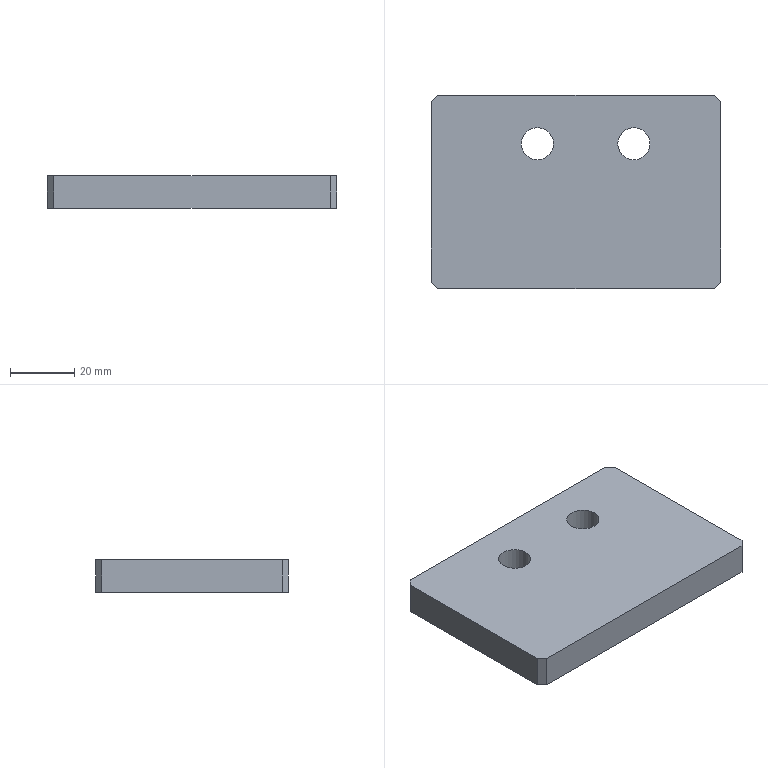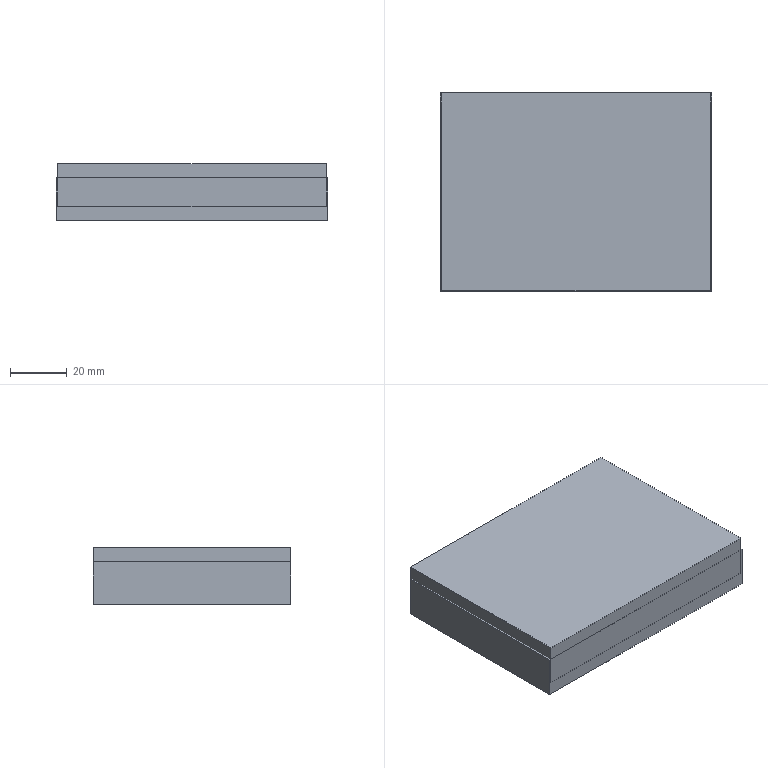CAM job | NX | 3-axis milling, drilling | part box 90 x 60 x 10 mm | stock box 96 x 70 x 20 mm
Tools:
number,name,description,diameter,corner_radius,flute_length,length,flutes
1,D80面刀,,80.0,0.0,50.0,75.0,2
2,D12开粗,,12.0,0.0,50.0,75.0,2
3,D10精光,,10.0,0.0,50.0,75.0,2
5,D6倒角刀,,6.0,0.0,50.0,75.0,2
6,D8.6钻头,,8.6,0.0,50.0,75.0,2
7,M10丝攻,,8.6,0.0,50.0,75.0,2
Operations:
program,operation,operation_type,tool,method,geometry_group,spindle_rpm,surface_speed,feed_per_tooth,feed_cut,feed_plunge,cut_length_mm,path_length_mm,cut_time_min,machine_time_min
G54,PLANAR_MILL,PlanarMilling,D80面刀,METHOD,G54,2000.0,502.0,0.2,800.0,100.0,180.0,215.9,0.225,0.2286
G54,ADAPTIVE_MILLING,CavityMilling,D12开粗,METHOD,WORKPIECE,3000.0,113.0,0.25,1500.0,100.0,3610.156,3666.156,1.991,1.996
G54,PLANAR_MILL_1,PlanarMilling,D10精光,METHOD,WORKPIECE,3000.0,94.0,0.1333,800.0,100.0,694.172,819.237,0.8677,0.8802
G54,SPOT_DRILLING,HoleDrilling,D6倒角刀,METHOD,WORKPIECE,2000.0,37.0,0.0375,150.0,100.0,16.0,114.0,0.1067,0.1165
G54,SPOT_DRILLING_COPY,HoleDrilling,D8.6钻头,METHOD,WORKPIECE,1600.0,43.0,0.0312,100.0,100.0,448.0,546.0,4.48,4.49
G54,PLANAR_MILL_1_COPY,PlanarMilling,D6倒角刀,METHOD,WORKPIECE,3000.0,94.0,0.1333,800.0,100.0,316.125,352.125,0.3952,0.3988
G54,PLANAR_MILL_1_COPY_COPY,PlanarMilling,D6倒角刀,METHOD,WORKPIECE,3000.0,94.0,0.1333,800.0,100.0,70.761,178.873,0.0885,0.0993
G54,SPOT_DRILLING_COPY_COPY,HoleDrilling,M10丝攻,METHOD,WORKPIECE,300.0,8.0,0.0025,1.5,100.0,60.0,158.0,40.0,40.01
G54,PLANAR_MILL_COPY,PlanarMilling,D80面刀,METHOD,G54,2000.0,502.0,0.2,800.0,100.0,180.0,216.0,0.225,0.2286
G55,ADAPTIVE_MILLING_COPY,CavityMilling,D12开粗,METHOD,WORKPIECE_1,3000.0,113.0,0.25,1500.0,100.0,13364.465,13398.265,8.91,8.913
G55,PLANAR_MILL_COPY_1,PlanarMilling,D80面刀,METHOD,G55,2000.0,502.0,0.2,800.0,100.0,180.0,215.9,0.225,0.2286
G55,PLANAR_MILL_2,PlanarMilling,D6倒角刀,METHOD,WORKPIECE_1,1061.0,100.0,0.1178,250.0,100.0,315.022,354.022,1.26,1.264
G55,PLANAR_MILL_2_COPY,PlanarMilling,D6倒角刀,METHOD,WORKPIECE_1,1061.0,100.0,0.1178,250.0,100.0,68.549,176.644,0.2742,0.285